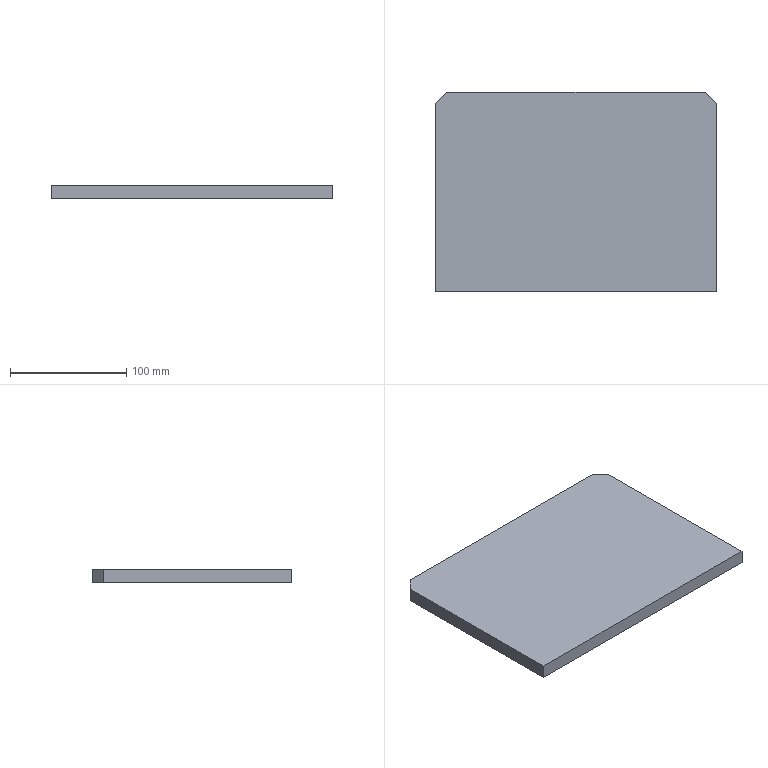Part | SolidWorks | features BaseBody 1 | 1 solid | 8 faces | box 242 x 172 x 12 mm | volume 498288 mm3 | plane 8
STEP:
#1=CARTESIAN_POINT('',(121.,-84.5,0.));
#2=VERTEX_POINT('',#1);
#3=CARTESIAN_POINT('',(121.,-84.5,12.));
#4=VERTEX_POINT('',#3);
#5=CARTESIAN_POINT('',(121.,-84.5,12.));
#6=DIRECTION('',(0.,0.,1.));
#7=VECTOR('',#6,1000.);
#8=LINE('',#5,#7);
#9=EDGE_CURVE('',#2,#4,#8,.T.);
#10=ORIENTED_EDGE('',*,*,#9,.F.);
#11=CARTESIAN_POINT('',(121.,77.5,0.));
#12=VERTEX_POINT('',#11);
#13=CARTESIAN_POINT('',(121.,77.5,0.));
#14=DIRECTION('',(0.,1.,0.));
#15=VECTOR('',#14,1000.);
#16=LINE('',#13,#15);
#17=EDGE_CURVE('',#2,#12,#16,.T.);
#18=ORIENTED_EDGE('',*,*,#17,.T.);
#19=CARTESIAN_POINT('',(121.,77.5,12.));
#20=VERTEX_POINT('',#19);
#21=CARTESIAN_POINT('',(121.,77.5,12.));
#22=DIRECTION('',(0.,0.,-1.));
#23=VECTOR('',#22,1000.);
#24=LINE('',#21,#23);
#25=EDGE_CURVE('',#20,#12,#24,.T.);
#26=ORIENTED_EDGE('',*,*,#25,.F.);
#27=CARTESIAN_POINT('',(121.,77.5,12.));
#28=DIRECTION('',(0.,1.,0.));
#29=VECTOR('',#28,1000.);
#30=LINE('',#27,#29);
#31=EDGE_CURVE('',#4,#20,#30,.T.);
#32=ORIENTED_EDGE('',*,*,#31,.F.);
#33=EDGE_LOOP('',(#10,#18,#26,#32));
#34=FACE_OUTER_BOUND('',#33,.T.);
#35=CARTESIAN_POINT('',(121.,77.5,12.));
#36=DIRECTION('',(-1.,0.,0.));
#37=DIRECTION('',(0.,-1.,0.));
#38=AXIS2_PLACEMENT_3D('',#35,#36,#37);
#39=PLANE('',#38);
#40=ADVANCED_FACE('',(#34),#39,.F.);
#41=CARTESIAN_POINT('',(-121.,-84.5,12.));
#42=VERTEX_POINT('',#41);
#43=CARTESIAN_POINT('',(-121.,-84.5,0.));
#44=VERTEX_POINT('',#43);
#45=CARTESIAN_POINT('',(-121.,-84.5,12.));
#46=DIRECTION('',(0.,0.,-1.));
#47=VECTOR('',#46,1000.);
#48=LINE('',#45,#47);
#49=EDGE_CURVE('',#42,#44,#48,.T.);
#50=ORIENTED_EDGE('',*,*,#49,.F.);
#51=CARTESIAN_POINT('',(-121.,77.5,12.));
#52=VERTEX_POINT('',#51);
#53=CARTESIAN_POINT('',(-121.,77.5,12.));
#54=DIRECTION('',(0.,-1.,0.));
#55=VECTOR('',#54,1000.);
#56=LINE('',#53,#55);
#57=EDGE_CURVE('',#52,#42,#56,.T.);
#58=ORIENTED_EDGE('',*,*,#57,.F.);
#59=CARTESIAN_POINT('',(-121.,77.5,0.));
#60=VERTEX_POINT('',#59);
#61=CARTESIAN_POINT('',(-121.,77.5,12.));
#62=DIRECTION('',(0.,0.,-1.));
#63=VECTOR('',#62,1000.);
#64=LINE('',#61,#63);
#65=EDGE_CURVE('',#52,#60,#64,.T.);
#66=ORIENTED_EDGE('',*,*,#65,.T.);
#67=CARTESIAN_POINT('',(-121.,77.5,0.));
#68=DIRECTION('',(0.,-1.,0.));
#69=VECTOR('',#68,1000.);
#70=LINE('',#67,#69);
#71=EDGE_CURVE('',#60,#44,#70,.T.);
#72=ORIENTED_EDGE('',*,*,#71,.T.);
#73=EDGE_LOOP('',(#50,#58,#66,#72));
#74=FACE_OUTER_BOUND('',#73,.T.);
#75=CARTESIAN_POINT('',(-121.,77.5,12.));
#76=DIRECTION('',(1.,0.,0.));
#77=DIRECTION('',(0.,1.,0.));
#78=AXIS2_PLACEMENT_3D('',#75,#76,#77);
#79=PLANE('',#78);
#80=ADVANCED_FACE('',(#74),#79,.F.);
#81=ORIENTED_EDGE('',*,*,#57,.T.);
#82=CARTESIAN_POINT('',(0.,-84.5,12.));
#83=DIRECTION('',(1.,0.,0.));
#84=VECTOR('',#83,1000.);
#85=LINE('',#82,#84);
#86=EDGE_CURVE('',#42,#4,#85,.T.);
#87=ORIENTED_EDGE('',*,*,#86,.T.);
#88=ORIENTED_EDGE('',*,*,#31,.T.);
#89=CARTESIAN_POINT('',(111.,87.5,12.));
#90=VERTEX_POINT('',#89);
#91=CARTESIAN_POINT('',(111.,87.5,12.));
#92=DIRECTION('',(-0.7071,0.7071,0.));
#93=VECTOR('',#92,1000.);
#94=LINE('',#91,#93);
#95=EDGE_CURVE('',#20,#90,#94,.T.);
#96=ORIENTED_EDGE('',*,*,#95,.T.);
#97=CARTESIAN_POINT('',(-111.,87.5,12.));
#98=VERTEX_POINT('',#97);
#99=CARTESIAN_POINT('',(-111.,87.5,12.));
#100=DIRECTION('',(-1.,0.,0.));
#101=VECTOR('',#100,1000.);
#102=LINE('',#99,#101);
#103=EDGE_CURVE('',#90,#98,#102,.T.);
#104=ORIENTED_EDGE('',*,*,#103,.T.);
#105=CARTESIAN_POINT('',(-121.,77.5,12.));
#106=DIRECTION('',(-0.7071,-0.7071,0.));
#107=VECTOR('',#106,1000.);
#108=LINE('',#105,#107);
#109=EDGE_CURVE('',#98,#52,#108,.T.);
#110=ORIENTED_EDGE('',*,*,#109,.T.);
#111=EDGE_LOOP('',(#81,#87,#88,#96,#104,#110));
#112=FACE_OUTER_BOUND('',#111,.T.);
#113=CARTESIAN_POINT('',(0.,0.,12.));
#114=DIRECTION('',(0.,0.,1.));
#115=DIRECTION('',(1.,0.,0.));
#116=AXIS2_PLACEMENT_3D('',#113,#114,#115);
#117=PLANE('',#116);
#118=ADVANCED_FACE('',(#112),#117,.T.);
#119=CARTESIAN_POINT('',(0.,-84.5,0.));
#120=DIRECTION('',(1.,0.,0.));
#121=VECTOR('',#120,1000.);
#122=LINE('',#119,#121);
#123=EDGE_CURVE('',#44,#2,#122,.T.);
#124=ORIENTED_EDGE('',*,*,#123,.F.);
#125=ORIENTED_EDGE('',*,*,#71,.F.);
#126=CARTESIAN_POINT('',(-111.,87.5,0.));
#127=VERTEX_POINT('',#126);
#128=CARTESIAN_POINT('',(-121.,77.5,0.));
#129=DIRECTION('',(-0.7071,-0.7071,0.));
#130=VECTOR('',#129,1000.);
#131=LINE('',#128,#130);
#132=EDGE_CURVE('',#127,#60,#131,.T.);
#133=ORIENTED_EDGE('',*,*,#132,.F.);
#134=CARTESIAN_POINT('',(111.,87.5,0.));
#135=VERTEX_POINT('',#134);
#136=CARTESIAN_POINT('',(-111.,87.5,0.));
#137=DIRECTION('',(-1.,0.,0.));
#138=VECTOR('',#137,1000.);
#139=LINE('',#136,#138);
#140=EDGE_CURVE('',#135,#127,#139,.T.);
#141=ORIENTED_EDGE('',*,*,#140,.F.);
#142=CARTESIAN_POINT('',(111.,87.5,0.));
#143=DIRECTION('',(-0.7071,0.7071,0.));
#144=VECTOR('',#143,1000.);
#145=LINE('',#142,#144);
#146=EDGE_CURVE('',#12,#135,#145,.T.);
#147=ORIENTED_EDGE('',*,*,#146,.F.);
#148=ORIENTED_EDGE('',*,*,#17,.F.);
#149=EDGE_LOOP('',(#124,#125,#133,#141,#147,#148));
#150=FACE_OUTER_BOUND('',#149,.T.);
#151=CARTESIAN_POINT('',(0.,0.,0.));
#152=DIRECTION('',(0.,0.,1.));
#153=DIRECTION('',(1.,0.,0.));
#154=AXIS2_PLACEMENT_3D('',#151,#152,#153);
#155=PLANE('',#154);
#156=ADVANCED_FACE('',(#150),#155,.F.);
#157=ORIENTED_EDGE('',*,*,#146,.T.);
#158=CARTESIAN_POINT('',(111.,87.5,12.));
#159=DIRECTION('',(0.,0.,-1.));
#160=VECTOR('',#159,1000.);
#161=LINE('',#158,#160);
#162=EDGE_CURVE('',#90,#135,#161,.T.);
#163=ORIENTED_EDGE('',*,*,#162,.F.);
#164=ORIENTED_EDGE('',*,*,#95,.F.);
#165=ORIENTED_EDGE('',*,*,#25,.T.);
#166=EDGE_LOOP('',(#157,#163,#164,#165));
#167=FACE_OUTER_BOUND('',#166,.T.);
#168=CARTESIAN_POINT('',(111.,87.5,12.));
#169=DIRECTION('',(-0.7071,-0.7071,0.));
#170=DIRECTION('',(0.7071,-0.7071,0.));
#171=AXIS2_PLACEMENT_3D('',#168,#169,#170);
#172=PLANE('',#171);
#173=ADVANCED_FACE('',(#167),#172,.F.);
#174=ORIENTED_EDGE('',*,*,#140,.T.);
#175=CARTESIAN_POINT('',(-111.,87.5,12.));
#176=DIRECTION('',(0.,0.,-1.));
#177=VECTOR('',#176,1000.);
#178=LINE('',#175,#177);
#179=EDGE_CURVE('',#98,#127,#178,.T.);
#180=ORIENTED_EDGE('',*,*,#179,.F.);
#181=ORIENTED_EDGE('',*,*,#103,.F.);
#182=ORIENTED_EDGE('',*,*,#162,.T.);
#183=EDGE_LOOP('',(#174,#180,#181,#182));
#184=FACE_OUTER_BOUND('',#183,.T.);
#185=CARTESIAN_POINT('',(-111.,87.5,12.));
#186=DIRECTION('',(0.,-1.,0.));
#187=DIRECTION('',(0.,0.,-1.));
#188=AXIS2_PLACEMENT_3D('',#185,#186,#187);
#189=PLANE('',#188);
#190=ADVANCED_FACE('',(#184),#189,.F.);
#191=ORIENTED_EDGE('',*,*,#132,.T.);
#192=ORIENTED_EDGE('',*,*,#65,.F.);
#193=ORIENTED_EDGE('',*,*,#109,.F.);
#194=ORIENTED_EDGE('',*,*,#179,.T.);
#195=EDGE_LOOP('',(#191,#192,#193,#194));
#196=FACE_OUTER_BOUND('',#195,.T.);
#197=CARTESIAN_POINT('',(-121.,77.5,12.));
#198=DIRECTION('',(0.7071,-0.7071,0.));
#199=DIRECTION('',(0.7071,0.7071,0.));
#200=AXIS2_PLACEMENT_3D('',#197,#198,#199);
#201=PLANE('',#200);
#202=ADVANCED_FACE('',(#196),#201,.F.);
#203=ORIENTED_EDGE('',*,*,#49,.T.);
#204=ORIENTED_EDGE('',*,*,#123,.T.);
#205=ORIENTED_EDGE('',*,*,#9,.T.);
#206=ORIENTED_EDGE('',*,*,#86,.F.);
#207=EDGE_LOOP('',(#203,#204,#205,#206));
#208=FACE_OUTER_BOUND('',#207,.T.);
#209=CARTESIAN_POINT('',(467.,-84.5,6.));
#210=DIRECTION('',(0.,-1.,0.));
#211=DIRECTION('',(0.,0.,-1.));
#212=AXIS2_PLACEMENT_3D('',#209,#210,#211);
#213=PLANE('',#212);
#214=ADVANCED_FACE('',(#208),#213,.T.);
#215=CLOSED_SHELL('',(#40,#80,#118,#156,#173,#190,#202,#214));
#216=MANIFOLD_SOLID_BREP('',#215);
#217=CARTESIAN_POINT('',(0.,0.,0.));
#218=DIRECTION('',(0.,0.,1.));
#219=DIRECTION('',(1.,0.,0.));
#220=AXIS2_PLACEMENT_3D('',#217,#218,#219);
#221=(LENGTH_UNIT()NAMED_UNIT(*)SI_UNIT(.MILLI.,.METRE.));
#222=UNCERTAINTY_MEASURE_WITH_UNIT(LENGTH_MEASURE(0.00001),#221,'','');
#223=(NAMED_UNIT(*)PLANE_ANGLE_UNIT()SI_UNIT($,.RADIAN.));
#224=(NAMED_UNIT(*)SI_UNIT($,.STERADIAN.)SOLID_ANGLE_UNIT());
#225=(GEOMETRIC_REPRESENTATION_CONTEXT(3)GLOBAL_UNCERTAINTY_ASSIGNED_CONTEXT((#222))GLOBAL_UNIT_ASSIGNED_CONTEXT((#221,#223,#224))REPRESENTATION_CONTEXT('',''));
#226=ADVANCED_BREP_SHAPE_REPRESENTATION('',(#216,#220),#225);